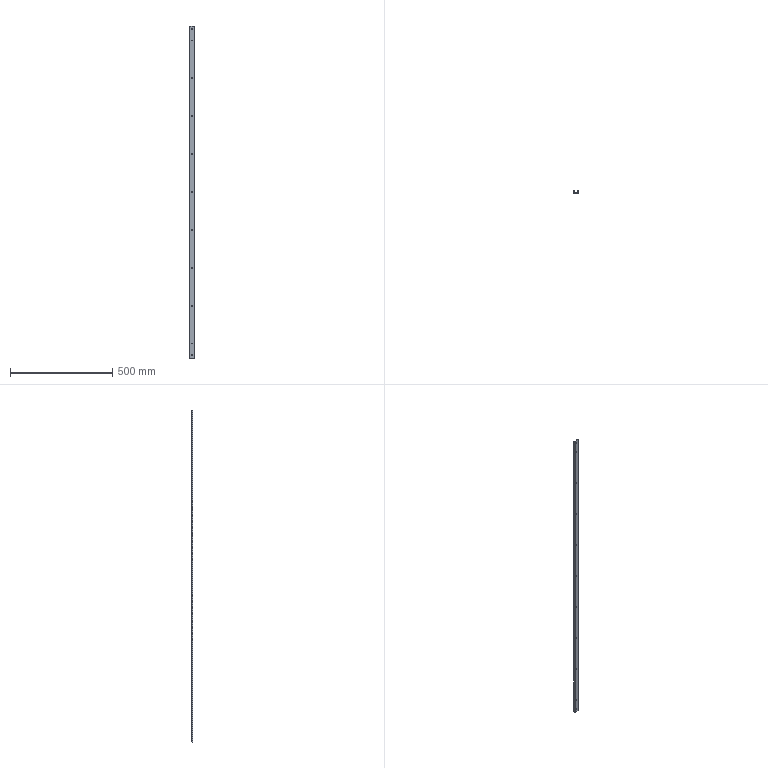Part | STEP file | 1 solid | 36 faces | box 20 x 8 x 1620 mm | volume 65186 mm3 | cylinder 26 | plane 10 | commonest cylinder face diameters 3.2 x22 10 x4